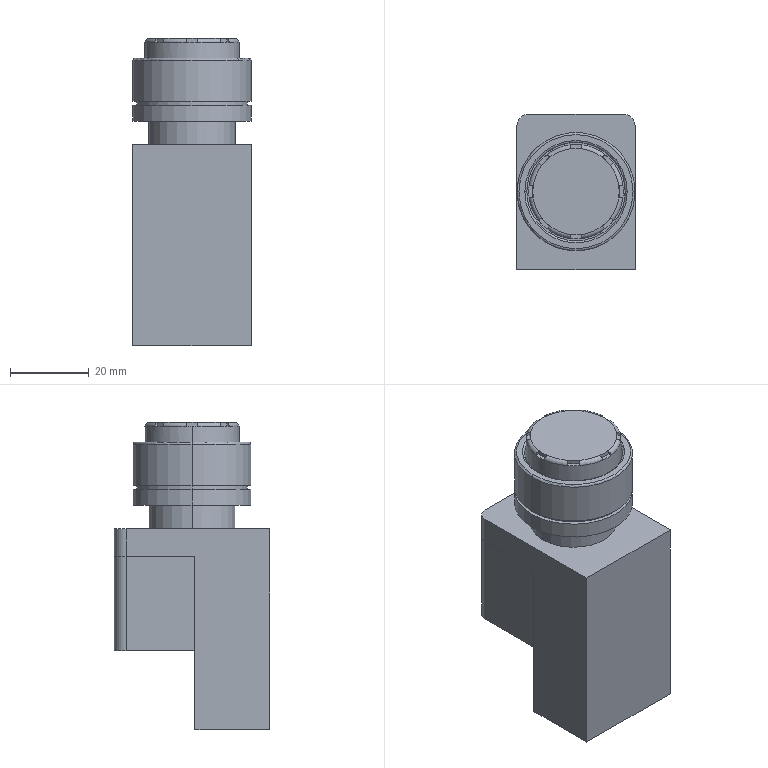Part | STEP file | Fuji Electric AR9T511-M | 3 solids | 85 faces | box 30 x 39.5 x 78 mm | volume 61141 mm3 | plane 57 | cylinder 16 | torus 12 | commonest cylinder face diameters 6 x4 30 x4 22 x2 24 x2 25 x2 28 x2